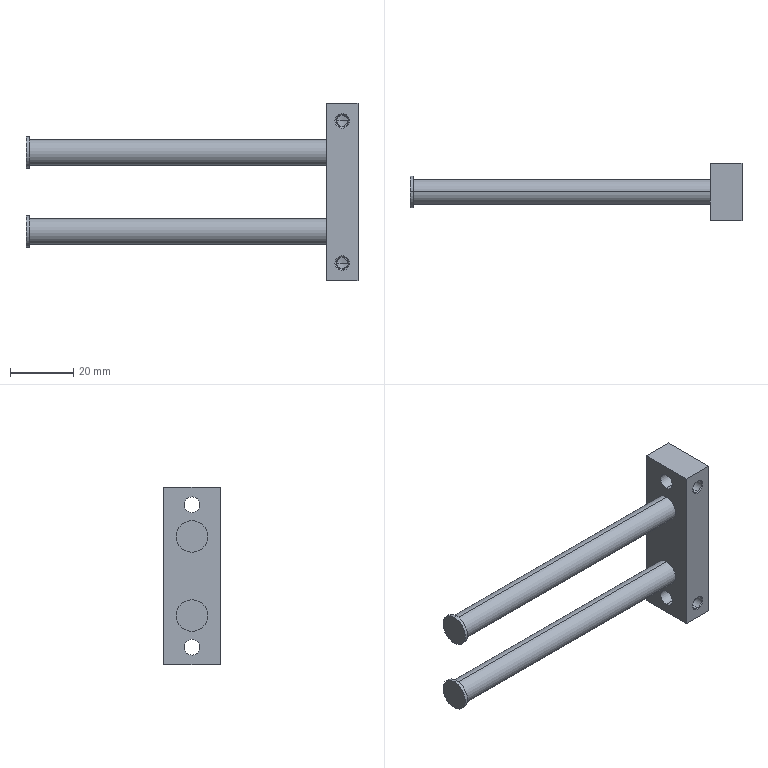Part | NX | 1 solid | 87 faces | box 105 x 18 x 56 mm | volume 18787 mm3 | cylinder 34 | plane 31 | cone 22 | commonest cylinder face diameters 3.4 x8 4 x8 5 x6 8 x4 10 x4 8.5 x2